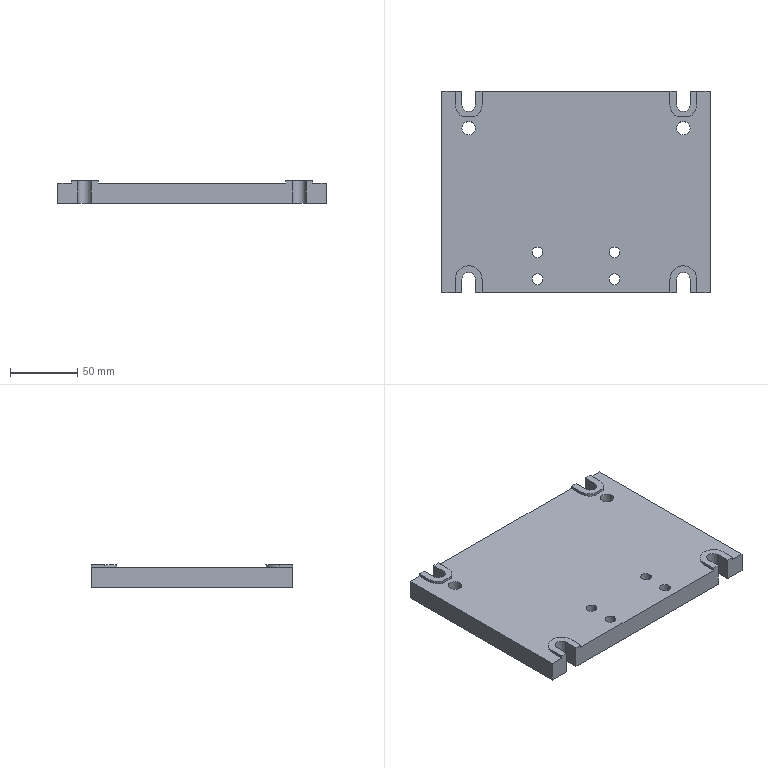Part | NX | features DATUM_CSYS 9, EXTRUDE 9, SKETCH 9, OFFSET_REGION 5, BREP 1, DELETE FACE 1 | 1 solid | 56 faces | box 200 x 150 x 17 mm | volume 435629 mm3 | plane 34 | cylinder 22 | commonest cylinder face diameters 8 x8 20 x8 10 x6